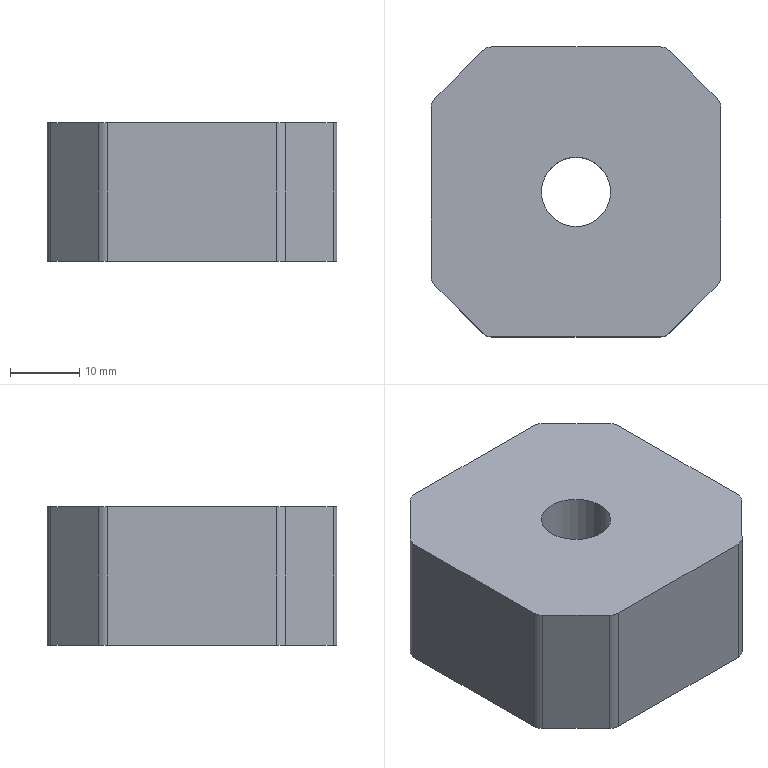Part | NX | 1 solid | 19 faces | box 41.814 x 41.814 x 20 mm | volume 30859 mm3 | plane 10 | cylinder 9 | commonest cylinder face diameters 3.814 x8 10 x1
STEP:
#1=CARTESIAN_POINT('',(-5.,0.,10.));
#2=VERTEX_POINT('',#1);
#3=CARTESIAN_POINT('',(0.,0.,10.));
#4=DIRECTION('',(0.,0.,-1.));
#5=DIRECTION('',(-1.,0.,0.));
#6=AXIS2_PLACEMENT_3D('',#3,#4,#5);
#7=CIRCLE('',#6,5.);
#8=EDGE_CURVE('',#2,#2,#7,.T.);
#9=ORIENTED_EDGE('',*,*,#8,.T.);
#10=EDGE_LOOP('',(#9));
#11=FACE_BOUND('',#10,.T.);
#12=CARTESIAN_POINT('',(-20.907,12.172,10.));
#13=VERTEX_POINT('',#12);
#14=CARTESIAN_POINT('',(-20.907,-12.172,10.));
#15=VERTEX_POINT('',#14);
#16=CARTESIAN_POINT('',(-20.907,0.,10.));
#17=DIRECTION('',(0.,1.,0.));
#18=VECTOR('',#17,1000.);
#19=LINE('',#16,#18);
#20=EDGE_CURVE('',#13,#15,#19,.F.);
#21=ORIENTED_EDGE('',*,*,#20,.T.);
#22=CARTESIAN_POINT('',(-20.348,-13.52,10.));
#23=VERTEX_POINT('',#22);
#24=CARTESIAN_POINT('',(-19.,-12.172,10.));
#25=DIRECTION('',(0.,0.,1.));
#26=DIRECTION('',(1.,0.,0.));
#27=AXIS2_PLACEMENT_3D('',#24,#25,#26);
#28=CIRCLE('',#27,1.907);
#29=EDGE_CURVE('',#23,#15,#28,.F.);
#30=ORIENTED_EDGE('',*,*,#29,.F.);
#31=CARTESIAN_POINT('',(-13.52,-20.348,10.));
#32=VERTEX_POINT('',#31);
#33=CARTESIAN_POINT('',(-20.348,-13.52,10.));
#34=DIRECTION('',(0.7071,-0.7071,0.));
#35=VECTOR('',#34,1000.);
#36=LINE('',#33,#35);
#37=EDGE_CURVE('',#23,#32,#36,.T.);
#38=ORIENTED_EDGE('',*,*,#37,.T.);
#39=CARTESIAN_POINT('',(-12.172,-20.907,10.));
#40=VERTEX_POINT('',#39);
#41=CARTESIAN_POINT('',(-12.172,-19.,10.));
#42=DIRECTION('',(0.,0.,1.));
#43=DIRECTION('',(1.,0.,0.));
#44=AXIS2_PLACEMENT_3D('',#41,#42,#43);
#45=CIRCLE('',#44,1.907);
#46=EDGE_CURVE('',#40,#32,#45,.F.);
#47=ORIENTED_EDGE('',*,*,#46,.F.);
#48=CARTESIAN_POINT('',(12.172,-20.907,10.));
#49=VERTEX_POINT('',#48);
#50=CARTESIAN_POINT('',(0.,-20.907,10.));
#51=DIRECTION('',(1.,0.,0.));
#52=VECTOR('',#51,1000.);
#53=LINE('',#50,#52);
#54=EDGE_CURVE('',#40,#49,#53,.T.);
#55=ORIENTED_EDGE('',*,*,#54,.T.);
#56=CARTESIAN_POINT('',(13.52,-20.348,10.));
#57=VERTEX_POINT('',#56);
#58=CARTESIAN_POINT('',(12.172,-19.,10.));
#59=DIRECTION('',(0.,0.,1.));
#60=DIRECTION('',(1.,0.,0.));
#61=AXIS2_PLACEMENT_3D('',#58,#59,#60);
#62=CIRCLE('',#61,1.907);
#63=EDGE_CURVE('',#57,#49,#62,.F.);
#64=ORIENTED_EDGE('',*,*,#63,.F.);
#65=CARTESIAN_POINT('',(20.348,-13.52,10.));
#66=VERTEX_POINT('',#65);
#67=CARTESIAN_POINT('',(13.52,-20.348,10.));
#68=DIRECTION('',(0.7071,0.7071,0.));
#69=VECTOR('',#68,1000.);
#70=LINE('',#67,#69);
#71=EDGE_CURVE('',#57,#66,#70,.T.);
#72=ORIENTED_EDGE('',*,*,#71,.T.);
#73=CARTESIAN_POINT('',(20.907,-12.172,10.));
#74=VERTEX_POINT('',#73);
#75=CARTESIAN_POINT('',(19.,-12.172,10.));
#76=DIRECTION('',(0.,0.,1.));
#77=DIRECTION('',(1.,0.,0.));
#78=AXIS2_PLACEMENT_3D('',#75,#76,#77);
#79=CIRCLE('',#78,1.907);
#80=EDGE_CURVE('',#74,#66,#79,.F.);
#81=ORIENTED_EDGE('',*,*,#80,.F.);
#82=CARTESIAN_POINT('',(20.907,12.172,10.));
#83=VERTEX_POINT('',#82);
#84=CARTESIAN_POINT('',(20.907,0.,10.));
#85=DIRECTION('',(0.,1.,0.));
#86=VECTOR('',#85,1000.);
#87=LINE('',#84,#86);
#88=EDGE_CURVE('',#74,#83,#87,.T.);
#89=ORIENTED_EDGE('',*,*,#88,.T.);
#90=CARTESIAN_POINT('',(20.348,13.52,10.));
#91=VERTEX_POINT('',#90);
#92=CARTESIAN_POINT('',(19.,12.172,10.));
#93=DIRECTION('',(0.,0.,1.));
#94=DIRECTION('',(1.,0.,0.));
#95=AXIS2_PLACEMENT_3D('',#92,#93,#94);
#96=CIRCLE('',#95,1.907);
#97=EDGE_CURVE('',#91,#83,#96,.F.);
#98=ORIENTED_EDGE('',*,*,#97,.F.);
#99=CARTESIAN_POINT('',(13.52,20.348,10.));
#100=VERTEX_POINT('',#99);
#101=CARTESIAN_POINT('',(20.348,13.52,10.));
#102=DIRECTION('',(-0.7071,0.7071,0.));
#103=VECTOR('',#102,1000.);
#104=LINE('',#101,#103);
#105=EDGE_CURVE('',#91,#100,#104,.T.);
#106=ORIENTED_EDGE('',*,*,#105,.T.);
#107=CARTESIAN_POINT('',(12.172,20.907,10.));
#108=VERTEX_POINT('',#107);
#109=CARTESIAN_POINT('',(12.172,19.,10.));
#110=DIRECTION('',(0.,0.,1.));
#111=DIRECTION('',(1.,0.,0.));
#112=AXIS2_PLACEMENT_3D('',#109,#110,#111);
#113=CIRCLE('',#112,1.907);
#114=EDGE_CURVE('',#108,#100,#113,.F.);
#115=ORIENTED_EDGE('',*,*,#114,.F.);
#116=CARTESIAN_POINT('',(-12.172,20.907,10.));
#117=VERTEX_POINT('',#116);
#118=CARTESIAN_POINT('',(0.,20.907,10.));
#119=DIRECTION('',(1.,0.,0.));
#120=VECTOR('',#119,1000.);
#121=LINE('',#118,#120);
#122=EDGE_CURVE('',#108,#117,#121,.F.);
#123=ORIENTED_EDGE('',*,*,#122,.T.);
#124=CARTESIAN_POINT('',(-13.52,20.348,10.));
#125=VERTEX_POINT('',#124);
#126=CARTESIAN_POINT('',(-12.172,19.,10.));
#127=DIRECTION('',(0.,0.,1.));
#128=DIRECTION('',(1.,0.,0.));
#129=AXIS2_PLACEMENT_3D('',#126,#127,#128);
#130=CIRCLE('',#129,1.907);
#131=EDGE_CURVE('',#125,#117,#130,.F.);
#132=ORIENTED_EDGE('',*,*,#131,.F.);
#133=CARTESIAN_POINT('',(-20.348,13.52,10.));
#134=VERTEX_POINT('',#133);
#135=CARTESIAN_POINT('',(-13.52,20.348,10.));
#136=DIRECTION('',(-0.7071,-0.7071,0.));
#137=VECTOR('',#136,1000.);
#138=LINE('',#135,#137);
#139=EDGE_CURVE('',#125,#134,#138,.T.);
#140=ORIENTED_EDGE('',*,*,#139,.T.);
#141=CARTESIAN_POINT('',(-19.,12.172,10.));
#142=DIRECTION('',(0.,0.,1.));
#143=DIRECTION('',(1.,0.,0.));
#144=AXIS2_PLACEMENT_3D('',#141,#142,#143);
#145=CIRCLE('',#144,1.907);
#146=EDGE_CURVE('',#13,#134,#145,.F.);
#147=ORIENTED_EDGE('',*,*,#146,.F.);
#148=EDGE_LOOP('',(#21,#30,#38,#47,#55,#64,#72,#81,#89,#98,#106,#115,#123,#132,#140,#147));
#149=FACE_BOUND('',#148,.T.);
#150=CARTESIAN_POINT('',(0.,0.,10.));
#151=DIRECTION('',(0.,0.,1.));
#152=DIRECTION('',(1.,0.,0.));
#153=AXIS2_PLACEMENT_3D('',#150,#151,#152);
#154=PLANE('',#153);
#155=ADVANCED_FACE('',(#11,#149),#154,.T.);
#156=ORIENTED_EDGE('',*,*,#8,.F.);
#157=EDGE_LOOP('',(#156));
#158=FACE_BOUND('',#157,.T.);
#159=CARTESIAN_POINT('',(-5.,0.,-10.));
#160=VERTEX_POINT('',#159);
#161=CARTESIAN_POINT('',(0.,0.,-10.));
#162=DIRECTION('',(0.,0.,-1.));
#163=DIRECTION('',(-1.,0.,0.));
#164=AXIS2_PLACEMENT_3D('',#161,#162,#163);
#165=CIRCLE('',#164,5.);
#166=EDGE_CURVE('',#160,#160,#165,.F.);
#167=ORIENTED_EDGE('',*,*,#166,.F.);
#168=EDGE_LOOP('',(#167));
#169=FACE_BOUND('',#168,.T.);
#170=CARTESIAN_POINT('',(0.,0.,10.));
#171=DIRECTION('',(0.,0.,-1.));
#172=DIRECTION('',(-1.,0.,0.));
#173=AXIS2_PLACEMENT_3D('',#170,#171,#172);
#174=CYLINDRICAL_SURFACE('',#173,5.);
#175=ADVANCED_FACE('',(#158,#169),#174,.F.);
#176=CARTESIAN_POINT('',(-20.907,12.172,-10.));
#177=VERTEX_POINT('',#176);
#178=CARTESIAN_POINT('',(-20.907,-12.172,-10.));
#179=VERTEX_POINT('',#178);
#180=CARTESIAN_POINT('',(-20.907,-12.172,-10.));
#181=DIRECTION('',(0.,1.,0.));
#182=VECTOR('',#181,1000.);
#183=LINE('',#180,#182);
#184=EDGE_CURVE('',#177,#179,#183,.F.);
#185=ORIENTED_EDGE('',*,*,#184,.T.);
#186=CARTESIAN_POINT('',(-20.907,-12.172,-10.));
#187=DIRECTION('',(0.,0.,1.));
#188=VECTOR('',#187,1000.);
#189=LINE('',#186,#188);
#190=EDGE_CURVE('',#179,#15,#189,.T.);
#191=ORIENTED_EDGE('',*,*,#190,.T.);
#192=ORIENTED_EDGE('',*,*,#20,.F.);
#193=CARTESIAN_POINT('',(-20.907,12.172,-10.));
#194=DIRECTION('',(0.,0.,1.));
#195=VECTOR('',#194,1000.);
#196=LINE('',#193,#195);
#197=EDGE_CURVE('',#13,#177,#196,.F.);
#198=ORIENTED_EDGE('',*,*,#197,.T.);
#199=EDGE_LOOP('',(#185,#191,#192,#198));
#200=FACE_BOUND('',#199,.T.);
#201=CARTESIAN_POINT('',(-20.907,-12.172,-10.));
#202=DIRECTION('',(-1.,0.,0.));
#203=DIRECTION('',(0.,0.,1.));
#204=AXIS2_PLACEMENT_3D('',#201,#202,#203);
#205=PLANE('',#204);
#206=ADVANCED_FACE('',(#200),#205,.T.);
#207=CARTESIAN_POINT('',(-13.52,20.348,-10.));
#208=VERTEX_POINT('',#207);
#209=CARTESIAN_POINT('',(-20.348,13.52,-10.));
#210=VERTEX_POINT('',#209);
#211=CARTESIAN_POINT('',(-20.348,13.52,-10.));
#212=DIRECTION('',(-0.7071,-0.7071,0.));
#213=VECTOR('',#212,1000.);
#214=LINE('',#211,#213);
#215=EDGE_CURVE('',#208,#210,#214,.T.);
#216=ORIENTED_EDGE('',*,*,#215,.T.);
#217=CARTESIAN_POINT('',(-20.348,13.52,-10.));
#218=DIRECTION('',(0.,0.,1.));
#219=VECTOR('',#218,1000.);
#220=LINE('',#217,#219);
#221=EDGE_CURVE('',#210,#134,#220,.T.);
#222=ORIENTED_EDGE('',*,*,#221,.T.);
#223=ORIENTED_EDGE('',*,*,#139,.F.);
#224=CARTESIAN_POINT('',(-13.52,20.348,-10.));
#225=DIRECTION('',(0.,0.,1.));
#226=VECTOR('',#225,1000.);
#227=LINE('',#224,#226);
#228=EDGE_CURVE('',#125,#208,#227,.F.);
#229=ORIENTED_EDGE('',*,*,#228,.T.);
#230=EDGE_LOOP('',(#216,#222,#223,#229));
#231=FACE_BOUND('',#230,.T.);
#232=CARTESIAN_POINT('',(-20.348,13.52,-10.));
#233=DIRECTION('',(-0.7071,0.7071,0.));
#234=DIRECTION('',(-0.7071,-0.7071,0.));
#235=AXIS2_PLACEMENT_3D('',#232,#233,#234);
#236=PLANE('',#235);
#237=ADVANCED_FACE('',(#231),#236,.T.);
#238=CARTESIAN_POINT('',(12.172,20.907,-10.));
#239=VERTEX_POINT('',#238);
#240=CARTESIAN_POINT('',(-12.172,20.907,-10.));
#241=VERTEX_POINT('',#240);
#242=CARTESIAN_POINT('',(-12.172,20.907,-10.));
#243=DIRECTION('',(1.,0.,0.));
#244=VECTOR('',#243,1000.);
#245=LINE('',#242,#244);
#246=EDGE_CURVE('',#239,#241,#245,.F.);
#247=ORIENTED_EDGE('',*,*,#246,.T.);
#248=CARTESIAN_POINT('',(-12.172,20.907,-10.));
#249=DIRECTION('',(0.,0.,1.));
#250=VECTOR('',#249,1000.);
#251=LINE('',#248,#250);
#252=EDGE_CURVE('',#241,#117,#251,.T.);
#253=ORIENTED_EDGE('',*,*,#252,.T.);
#254=ORIENTED_EDGE('',*,*,#122,.F.);
#255=CARTESIAN_POINT('',(12.172,20.907,-10.));
#256=DIRECTION('',(0.,0.,1.));
#257=VECTOR('',#256,1000.);
#258=LINE('',#255,#257);
#259=EDGE_CURVE('',#108,#239,#258,.F.);
#260=ORIENTED_EDGE('',*,*,#259,.T.);
#261=EDGE_LOOP('',(#247,#253,#254,#260));
#262=FACE_BOUND('',#261,.T.);
#263=CARTESIAN_POINT('',(-12.172,20.907,-10.));
#264=DIRECTION('',(0.,1.,0.));
#265=DIRECTION('',(0.,0.,1.));
#266=AXIS2_PLACEMENT_3D('',#263,#264,#265);
#267=PLANE('',#266);
#268=ADVANCED_FACE('',(#262),#267,.T.);
#269=CARTESIAN_POINT('',(20.348,13.52,-10.));
#270=VERTEX_POINT('',#269);
#271=CARTESIAN_POINT('',(13.52,20.348,-10.));
#272=VERTEX_POINT('',#271);
#273=CARTESIAN_POINT('',(13.52,20.348,-10.));
#274=DIRECTION('',(-0.7071,0.7071,0.));
#275=VECTOR('',#274,1000.);
#276=LINE('',#273,#275);
#277=EDGE_CURVE('',#270,#272,#276,.T.);
#278=ORIENTED_EDGE('',*,*,#277,.T.);
#279=CARTESIAN_POINT('',(13.52,20.348,-10.));
#280=DIRECTION('',(0.,0.,1.));
#281=VECTOR('',#280,1000.);
#282=LINE('',#279,#281);
#283=EDGE_CURVE('',#272,#100,#282,.T.);
#284=ORIENTED_EDGE('',*,*,#283,.T.);
#285=ORIENTED_EDGE('',*,*,#105,.F.);
#286=CARTESIAN_POINT('',(20.348,13.52,-10.));
#287=DIRECTION('',(0.,0.,1.));
#288=VECTOR('',#287,1000.);
#289=LINE('',#286,#288);
#290=EDGE_CURVE('',#91,#270,#289,.F.);
#291=ORIENTED_EDGE('',*,*,#290,.T.);
#292=EDGE_LOOP('',(#278,#284,#285,#291));
#293=FACE_BOUND('',#292,.T.);
#294=CARTESIAN_POINT('',(13.52,20.348,-10.));
#295=DIRECTION('',(0.7071,0.7071,0.));
#296=DIRECTION('',(-0.7071,0.7071,0.));
#297=AXIS2_PLACEMENT_3D('',#294,#295,#296);
#298=PLANE('',#297);
#299=ADVANCED_FACE('',(#293),#298,.T.);
#300=CARTESIAN_POINT('',(20.907,-12.172,-10.));
#301=VERTEX_POINT('',#300);
#302=CARTESIAN_POINT('',(20.907,12.172,-10.));
#303=VERTEX_POINT('',#302);
#304=CARTESIAN_POINT('',(20.907,12.172,-10.));
#305=DIRECTION('',(0.,1.,0.));
#306=VECTOR('',#305,1000.);
#307=LINE('',#304,#306);
#308=EDGE_CURVE('',#301,#303,#307,.T.);
#309=ORIENTED_EDGE('',*,*,#308,.T.);
#310=CARTESIAN_POINT('',(20.907,12.172,-10.));
#311=DIRECTION('',(0.,0.,-1.));
#312=VECTOR('',#311,1000.);
#313=LINE('',#310,#312);
#314=EDGE_CURVE('',#303,#83,#313,.F.);
#315=ORIENTED_EDGE('',*,*,#314,.T.);
#316=ORIENTED_EDGE('',*,*,#88,.F.);
#317=CARTESIAN_POINT('',(20.907,-12.172,-10.));
#318=DIRECTION('',(0.,0.,-1.));
#319=VECTOR('',#318,1000.);
#320=LINE('',#317,#319);
#321=EDGE_CURVE('',#74,#301,#320,.T.);
#322=ORIENTED_EDGE('',*,*,#321,.T.);
#323=EDGE_LOOP('',(#309,#315,#316,#322));
#324=FACE_BOUND('',#323,.T.);
#325=CARTESIAN_POINT('',(20.907,12.172,-10.));
#326=DIRECTION('',(1.,0.,0.));
#327=DIRECTION('',(0.,0.,-1.));
#328=AXIS2_PLACEMENT_3D('',#325,#326,#327);
#329=PLANE('',#328);
#330=ADVANCED_FACE('',(#324),#329,.T.);
#331=CARTESIAN_POINT('',(13.52,-20.348,-10.));
#332=VERTEX_POINT('',#331);
#333=CARTESIAN_POINT('',(20.348,-13.52,-10.));
#334=VERTEX_POINT('',#333);
#335=CARTESIAN_POINT('',(20.348,-13.52,-10.));
#336=DIRECTION('',(0.7071,0.7071,0.));
#337=VECTOR('',#336,1000.);
#338=LINE('',#335,#337);
#339=EDGE_CURVE('',#332,#334,#338,.T.);
#340=ORIENTED_EDGE('',*,*,#339,.T.);
#341=CARTESIAN_POINT('',(20.348,-13.52,-10.));
#342=DIRECTION('',(0.,0.,1.));
#343=VECTOR('',#342,1000.);
#344=LINE('',#341,#343);
#345=EDGE_CURVE('',#334,#66,#344,.T.);
#346=ORIENTED_EDGE('',*,*,#345,.T.);
#347=ORIENTED_EDGE('',*,*,#71,.F.);
#348=CARTESIAN_POINT('',(13.52,-20.348,-10.));
#349=DIRECTION('',(0.,0.,1.));
#350=VECTOR('',#349,1000.);
#351=LINE('',#348,#350);
#352=EDGE_CURVE('',#57,#332,#351,.F.);
#353=ORIENTED_EDGE('',*,*,#352,.T.);
#354=EDGE_LOOP('',(#340,#346,#347,#353));
#355=FACE_BOUND('',#354,.T.);
#356=CARTESIAN_POINT('',(20.348,-13.52,-10.));
#357=DIRECTION('',(0.7071,-0.7071,0.));
#358=DIRECTION('',(0.7071,0.7071,0.));
#359=AXIS2_PLACEMENT_3D('',#356,#357,#358);
#360=PLANE('',#359);
#361=ADVANCED_FACE('',(#355),#360,.T.);
#362=CARTESIAN_POINT('',(-12.172,-20.907,-10.));
#363=VERTEX_POINT('',#362);
#364=CARTESIAN_POINT('',(12.172,-20.907,-10.));
#365=VERTEX_POINT('',#364);
#366=CARTESIAN_POINT('',(12.172,-20.907,-10.));
#367=DIRECTION('',(1.,0.,0.));
#368=VECTOR('',#367,1000.);
#369=LINE('',#366,#368);
#370=EDGE_CURVE('',#363,#365,#369,.T.);
#371=ORIENTED_EDGE('',*,*,#370,.T.);
#372=CARTESIAN_POINT('',(12.172,-20.907,-10.));
#373=DIRECTION('',(0.,0.,-1.));
#374=VECTOR('',#373,1000.);
#375=LINE('',#372,#374);
#376=EDGE_CURVE('',#365,#49,#375,.F.);
#377=ORIENTED_EDGE('',*,*,#376,.T.);
#378=ORIENTED_EDGE('',*,*,#54,.F.);
#379=CARTESIAN_POINT('',(-12.172,-20.907,-10.));
#380=DIRECTION('',(0.,0.,-1.));
#381=VECTOR('',#380,1000.);
#382=LINE('',#379,#381);
#383=EDGE_CURVE('',#40,#363,#382,.T.);
#384=ORIENTED_EDGE('',*,*,#383,.T.);
#385=EDGE_LOOP('',(#371,#377,#378,#384));
#386=FACE_BOUND('',#385,.T.);
#387=CARTESIAN_POINT('',(12.172,-20.907,-10.));
#388=DIRECTION('',(0.,-1.,0.));
#389=DIRECTION('',(0.,0.,-1.));
#390=AXIS2_PLACEMENT_3D('',#387,#388,#389);
#391=PLANE('',#390);
#392=ADVANCED_FACE('',(#386),#391,.T.);
#393=CARTESIAN_POINT('',(-20.348,-13.52,-10.));
#394=VERTEX_POINT('',#393);
#395=CARTESIAN_POINT('',(-13.52,-20.348,-10.));
#396=VERTEX_POINT('',#395);
#397=CARTESIAN_POINT('',(-13.52,-20.348,-10.));
#398=DIRECTION('',(0.7071,-0.7071,0.));
#399=VECTOR('',#398,1000.);
#400=LINE('',#397,#399);
#401=EDGE_CURVE('',#394,#396,#400,.T.);
#402=ORIENTED_EDGE('',*,*,#401,.T.);
#403=CARTESIAN_POINT('',(-13.52,-20.348,-10.));
#404=DIRECTION('',(0.,0.,1.));
#405=VECTOR('',#404,1000.);
#406=LINE('',#403,#405);
#407=EDGE_CURVE('',#396,#32,#406,.T.);
#408=ORIENTED_EDGE('',*,*,#407,.T.);
#409=ORIENTED_EDGE('',*,*,#37,.F.);
#410=CARTESIAN_POINT('',(-20.348,-13.52,-10.));
#411=DIRECTION('',(0.,0.,1.));
#412=VECTOR('',#411,1000.);
#413=LINE('',#410,#412);
#414=EDGE_CURVE('',#23,#394,#413,.F.);
#415=ORIENTED_EDGE('',*,*,#414,.T.);
#416=EDGE_LOOP('',(#402,#408,#409,#415));
#417=FACE_BOUND('',#416,.T.);
#418=CARTESIAN_POINT('',(-13.52,-20.348,-10.));
#419=DIRECTION('',(-0.7071,-0.7071,0.));
#420=DIRECTION('',(0.7071,-0.7071,0.));
#421=AXIS2_PLACEMENT_3D('',#418,#419,#420);
#422=PLANE('',#421);
#423=ADVANCED_FACE('',(#417),#422,.T.);
#424=ORIENTED_EDGE('',*,*,#166,.T.);
#425=EDGE_LOOP('',(#424));
#426=FACE_BOUND('',#425,.T.);
#427=CARTESIAN_POINT('',(-19.,-12.172,-10.));
#428=DIRECTION('',(0.,0.,1.));
#429=DIRECTION('',(1.,0.,0.));
#430=AXIS2_PLACEMENT_3D('',#427,#428,#429);
#431=CIRCLE('',#430,1.907);
#432=EDGE_CURVE('',#179,#394,#431,.T.);
#433=ORIENTED_EDGE('',*,*,#432,.F.);
#434=ORIENTED_EDGE('',*,*,#184,.F.);
#435=CARTESIAN_POINT('',(-19.,12.172,-10.));
#436=DIRECTION('',(0.,0.,1.));
#437=DIRECTION('',(1.,0.,0.));
#438=AXIS2_PLACEMENT_3D('',#435,#436,#437);
#439=CIRCLE('',#438,1.907);
#440=EDGE_CURVE('',#210,#177,#439,.T.);
#441=ORIENTED_EDGE('',*,*,#440,.F.);
#442=ORIENTED_EDGE('',*,*,#215,.F.);
#443=CARTESIAN_POINT('',(-12.172,19.,-10.));
#444=DIRECTION('',(0.,0.,1.));
#445=DIRECTION('',(1.,0.,0.));
#446=AXIS2_PLACEMENT_3D('',#443,#444,#445);
#447=CIRCLE('',#446,1.907);
#448=EDGE_CURVE('',#241,#208,#447,.T.);
#449=ORIENTED_EDGE('',*,*,#448,.F.);
#450=ORIENTED_EDGE('',*,*,#246,.F.);
#451=CARTESIAN_POINT('',(12.172,19.,-10.));
#452=DIRECTION('',(0.,0.,1.));
#453=DIRECTION('',(1.,0.,0.));
#454=AXIS2_PLACEMENT_3D('',#451,#452,#453);
#455=CIRCLE('',#454,1.907);
#456=EDGE_CURVE('',#272,#239,#455,.T.);
#457=ORIENTED_EDGE('',*,*,#456,.F.);
#458=ORIENTED_EDGE('',*,*,#277,.F.);
#459=CARTESIAN_POINT('',(19.,12.172,-10.));
#460=DIRECTION('',(0.,0.,1.));
#461=DIRECTION('',(1.,0.,0.));
#462=AXIS2_PLACEMENT_3D('',#459,#460,#461);
#463=CIRCLE('',#462,1.907);
#464=EDGE_CURVE('',#303,#270,#463,.T.);
#465=ORIENTED_EDGE('',*,*,#464,.F.);
#466=ORIENTED_EDGE('',*,*,#308,.F.);
#467=CARTESIAN_POINT('',(19.,-12.172,-10.));
#468=DIRECTION('',(0.,0.,1.));
#469=DIRECTION('',(1.,0.,0.));
#470=AXIS2_PLACEMENT_3D('',#467,#468,#469);
#471=CIRCLE('',#470,1.907);
#472=EDGE_CURVE('',#334,#301,#471,.T.);
#473=ORIENTED_EDGE('',*,*,#472,.F.);
#474=ORIENTED_EDGE('',*,*,#339,.F.);
#475=CARTESIAN_POINT('',(12.172,-19.,-10.));
#476=DIRECTION('',(0.,0.,1.));
#477=DIRECTION('',(1.,0.,0.));
#478=AXIS2_PLACEMENT_3D('',#475,#476,#477);
#479=CIRCLE('',#478,1.907);
#480=EDGE_CURVE('',#365,#332,#479,.T.);
#481=ORIENTED_EDGE('',*,*,#480,.F.);
#482=ORIENTED_EDGE('',*,*,#370,.F.);
#483=CARTESIAN_POINT('',(-12.172,-19.,-10.));
#484=DIRECTION('',(0.,0.,1.));
#485=DIRECTION('',(1.,0.,0.));
#486=AXIS2_PLACEMENT_3D('',#483,#484,#485);
#487=CIRCLE('',#486,1.907);
#488=EDGE_CURVE('',#396,#363,#487,.T.);
#489=ORIENTED_EDGE('',*,*,#488,.F.);
#490=ORIENTED_EDGE('',*,*,#401,.F.);
#491=EDGE_LOOP('',(#433,#434,#441,#442,#449,#450,#457,#458,#465,#466,#473,#474,#481,#482,#489,#490));
#492=FACE_BOUND('',#491,.T.);
#493=CARTESIAN_POINT('',(0.,0.,-10.));
#494=DIRECTION('',(0.,0.,1.));
#495=DIRECTION('',(1.,0.,0.));
#496=AXIS2_PLACEMENT_3D('',#493,#494,#495);
#497=PLANE('',#496);
#498=ADVANCED_FACE('',(#426,#492),#497,.F.);
#499=ORIENTED_EDGE('',*,*,#432,.T.);
#500=ORIENTED_EDGE('',*,*,#414,.F.);
#501=ORIENTED_EDGE('',*,*,#29,.T.);
#502=ORIENTED_EDGE('',*,*,#190,.F.);
#503=EDGE_LOOP('',(#499,#500,#501,#502));
#504=FACE_BOUND('',#503,.T.);
#505=CARTESIAN_POINT('',(-19.,-12.172,-10.));
#506=DIRECTION('',(0.,0.,1.));
#507=DIRECTION('',(1.,0.,0.));
#508=AXIS2_PLACEMENT_3D('',#505,#506,#507);
#509=CYLINDRICAL_SURFACE('',#508,1.907);
#510=ADVANCED_FACE('',(#504),#509,.T.);
#511=ORIENTED_EDGE('',*,*,#440,.T.);
#512=ORIENTED_EDGE('',*,*,#197,.F.);
#513=ORIENTED_EDGE('',*,*,#146,.T.);
#514=ORIENTED_EDGE('',*,*,#221,.F.);
#515=EDGE_LOOP('',(#511,#512,#513,#514));
#516=FACE_BOUND('',#515,.T.);
#517=CARTESIAN_POINT('',(-19.,12.172,-10.));
#518=DIRECTION('',(0.,0.,1.));
#519=DIRECTION('',(1.,0.,0.));
#520=AXIS2_PLACEMENT_3D('',#517,#518,#519);
#521=CYLINDRICAL_SURFACE('',#520,1.907);
#522=ADVANCED_FACE('',(#516),#521,.T.);
#523=ORIENTED_EDGE('',*,*,#448,.T.);
#524=ORIENTED_EDGE('',*,*,#228,.F.);
#525=ORIENTED_EDGE('',*,*,#131,.T.);
#526=ORIENTED_EDGE('',*,*,#252,.F.);
#527=EDGE_LOOP('',(#523,#524,#525,#526));
#528=FACE_BOUND('',#527,.T.);
#529=CARTESIAN_POINT('',(-12.172,19.,-10.));
#530=DIRECTION('',(0.,0.,1.));
#531=DIRECTION('',(1.,0.,0.));
#532=AXIS2_PLACEMENT_3D('',#529,#530,#531);
#533=CYLINDRICAL_SURFACE('',#532,1.907);
#534=ADVANCED_FACE('',(#528),#533,.T.);
#535=ORIENTED_EDGE('',*,*,#456,.T.);
#536=ORIENTED_EDGE('',*,*,#259,.F.);
#537=ORIENTED_EDGE('',*,*,#114,.T.);
#538=ORIENTED_EDGE('',*,*,#283,.F.);
#539=EDGE_LOOP('',(#535,#536,#537,#538));
#540=FACE_BOUND('',#539,.T.);
#541=CARTESIAN_POINT('',(12.172,19.,-10.));
#542=DIRECTION('',(0.,0.,1.));
#543=DIRECTION('',(1.,0.,0.));
#544=AXIS2_PLACEMENT_3D('',#541,#542,#543);
#545=CYLINDRICAL_SURFACE('',#544,1.907);
#546=ADVANCED_FACE('',(#540),#545,.T.);
#547=ORIENTED_EDGE('',*,*,#464,.T.);
#548=ORIENTED_EDGE('',*,*,#290,.F.);
#549=ORIENTED_EDGE('',*,*,#97,.T.);
#550=ORIENTED_EDGE('',*,*,#314,.F.);
#551=EDGE_LOOP('',(#547,#548,#549,#550));
#552=FACE_BOUND('',#551,.T.);
#553=CARTESIAN_POINT('',(19.,12.172,-10.));
#554=DIRECTION('',(0.,0.,1.));
#555=DIRECTION('',(1.,0.,0.));
#556=AXIS2_PLACEMENT_3D('',#553,#554,#555);
#557=CYLINDRICAL_SURFACE('',#556,1.907);
#558=ADVANCED_FACE('',(#552),#557,.T.);
#559=ORIENTED_EDGE('',*,*,#472,.T.);
#560=ORIENTED_EDGE('',*,*,#321,.F.);
#561=ORIENTED_EDGE('',*,*,#80,.T.);
#562=ORIENTED_EDGE('',*,*,#345,.F.);
#563=EDGE_LOOP('',(#559,#560,#561,#562));
#564=FACE_BOUND('',#563,.T.);
#565=CARTESIAN_POINT('',(19.,-12.172,-10.));
#566=DIRECTION('',(0.,0.,1.));
#567=DIRECTION('',(1.,0.,0.));
#568=AXIS2_PLACEMENT_3D('',#565,#566,#567);
#569=CYLINDRICAL_SURFACE('',#568,1.907);
#570=ADVANCED_FACE('',(#564),#569,.T.);
#571=ORIENTED_EDGE('',*,*,#480,.T.);
#572=ORIENTED_EDGE('',*,*,#352,.F.);
#573=ORIENTED_EDGE('',*,*,#63,.T.);
#574=ORIENTED_EDGE('',*,*,#376,.F.);
#575=EDGE_LOOP('',(#571,#572,#573,#574));
#576=FACE_BOUND('',#575,.T.);
#577=CARTESIAN_POINT('',(12.172,-19.,-10.));
#578=DIRECTION('',(0.,0.,1.));
#579=DIRECTION('',(1.,0.,0.));
#580=AXIS2_PLACEMENT_3D('',#577,#578,#579);
#581=CYLINDRICAL_SURFACE('',#580,1.907);
#582=ADVANCED_FACE('',(#576),#581,.T.);
#583=ORIENTED_EDGE('',*,*,#488,.T.);
#584=ORIENTED_EDGE('',*,*,#383,.F.);
#585=ORIENTED_EDGE('',*,*,#46,.T.);
#586=ORIENTED_EDGE('',*,*,#407,.F.);
#587=EDGE_LOOP('',(#583,#584,#585,#586));
#588=FACE_BOUND('',#587,.T.);
#589=CARTESIAN_POINT('',(-12.172,-19.,-10.));
#590=DIRECTION('',(0.,0.,1.));
#591=DIRECTION('',(1.,0.,0.));
#592=AXIS2_PLACEMENT_3D('',#589,#590,#591);
#593=CYLINDRICAL_SURFACE('',#592,1.907);
#594=ADVANCED_FACE('',(#588),#593,.T.);
#595=CLOSED_SHELL('',(#155,#175,#206,#237,#268,#299,#330,#361,#392,#423,#498,#510,#522,#534,#546,#558,#570,#582,#594));
#596=MANIFOLD_SOLID_BREP('',#595);
#597=(LENGTH_UNIT()NAMED_UNIT(*)SI_UNIT(.MILLI.,.METRE.));
#598=UNCERTAINTY_MEASURE_WITH_UNIT(LENGTH_MEASURE(0.00001),#597,'','');
#599=(NAMED_UNIT(*)PLANE_ANGLE_UNIT()SI_UNIT($,.RADIAN.));
#600=(NAMED_UNIT(*)SI_UNIT($,.STERADIAN.)SOLID_ANGLE_UNIT());
#601=(GEOMETRIC_REPRESENTATION_CONTEXT(3)GLOBAL_UNCERTAINTY_ASSIGNED_CONTEXT((#598))GLOBAL_UNIT_ASSIGNED_CONTEXT((#597,#599,#600))REPRESENTATION_CONTEXT('',''));
#602=ADVANCED_BREP_SHAPE_REPRESENTATION('',(#596),#601);